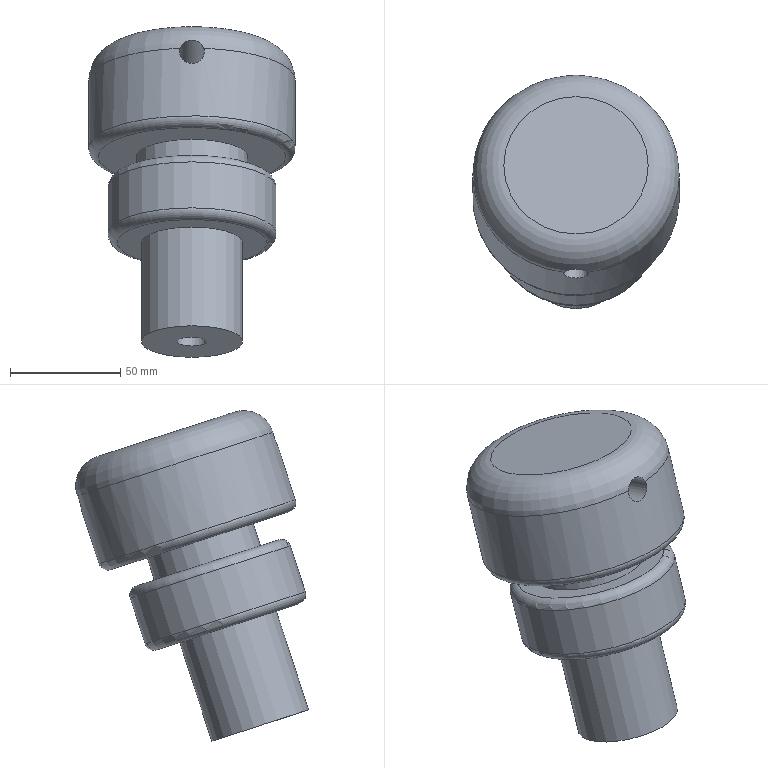Part | NX | features LINKED_BODY 2, DATUM_CSYS 1, Delete Body 1, Resize Face 1 | 1 solid | 19 faces | box 93.696 x 105.756 x 150.047 mm | volume 549540 mm3 | cylinder 9 | plane 6 | torus 4 | commonest cylinder face diameters 13.187 x3 11.25 x2 46.132 x1 50.625 x1 76.469 x1 93.696 x1
STEP:
#1=CARTESIAN_POINT('',(11.25,2935.24,-228.676));
#2=VERTEX_POINT('',#1);
#3=CARTESIAN_POINT('',(11.25,2941.511,-230.713));
#4=DIRECTION('',(0.,0.309,0.9511));
#5=DIRECTION('',(0.,-0.9511,0.309));
#6=AXIS2_PLACEMENT_3D('',#3,#4,#5);
#7=CIRCLE('',#6,6.594);
#8=EDGE_CURVE('',#2,#2,#7,.T.);
#9=ORIENTED_EDGE('',*,*,#8,.F.);
#10=EDGE_LOOP('',(#9));
#11=FACE_BOUND('',#10,.T.);
#12=CARTESIAN_POINT('',(16.87,2976.373,-112.26));
#13=VERTEX_POINT('',#12);
#14=CARTESIAN_POINT('',(5.63,2976.373,-112.26));
#15=VERTEX_POINT('',#14);
#16=CARTESIAN_POINT('',(16.87,2976.373,-112.26));
#17=CARTESIAN_POINT('',(16.904,2976.174,-113.052));
#18=CARTESIAN_POINT('',(16.6,2975.172,-114.385));
#19=CARTESIAN_POINT('',(15.455,2973.427,-115.676));
#20=CARTESIAN_POINT('',(13.683,2971.995,-116.606));
#21=CARTESIAN_POINT('',(11.25,2971.36,-116.988));
#22=CARTESIAN_POINT('',(8.831,2971.988,-116.61));
#23=CARTESIAN_POINT('',(7.045,2973.426,-115.676));
#24=CARTESIAN_POINT('',(5.901,2975.17,-114.39));
#25=CARTESIAN_POINT('',(5.596,2976.175,-113.047));
#26=CARTESIAN_POINT('',(5.63,2976.373,-112.26));
#27=B_SPLINE_CURVE_WITH_KNOTS('',3,(#16,#17,#18,#19,#20,#21,#22,#23,#24,#25,#26),.UNSPECIFIED.,.F.,.F.,(4,1,1,1,1,1,1,1,4),(0.006959,0.009375,0.01179,0.01421,0.01662,0.01904,0.02145,0.02387,0.02629),.UNSPECIFIED.);
#28=EDGE_CURVE('',#13,#15,#27,.T.);
#29=ORIENTED_EDGE('',*,*,#28,.F.);
#30=CARTESIAN_POINT('',(16.87,2982.932,-114.391));
#31=VERTEX_POINT('',#30);
#32=CARTESIAN_POINT('',(11.25,2979.653,-113.326));
#33=DIRECTION('',(0.,0.309,0.9511));
#34=DIRECTION('',(0.,-0.9511,0.309));
#35=AXIS2_PLACEMENT_3D('',#32,#33,#34);
#36=CIRCLE('',#35,6.594);
#37=EDGE_CURVE('',#13,#31,#36,.T.);
#38=ORIENTED_EDGE('',*,*,#37,.T.);
#39=CARTESIAN_POINT('',(5.63,2982.932,-114.391));
#40=VERTEX_POINT('',#39);
#41=CARTESIAN_POINT('',(5.63,2982.932,-114.391));
#42=CARTESIAN_POINT('',(5.596,2982.627,-115.149));
#43=CARTESIAN_POINT('',(5.9,2982.654,-116.816));
#44=CARTESIAN_POINT('',(7.045,2983.308,-118.887));
#45=CARTESIAN_POINT('',(8.817,2983.92,-120.481));
#46=CARTESIAN_POINT('',(11.25,2984.208,-121.163));
#47=CARTESIAN_POINT('',(13.669,2983.922,-120.488));
#48=CARTESIAN_POINT('',(15.455,2983.309,-118.887));
#49=CARTESIAN_POINT('',(16.599,2982.654,-116.822));
#50=CARTESIAN_POINT('',(16.904,2982.63,-115.144));
#51=CARTESIAN_POINT('',(16.87,2982.932,-114.391));
#52=B_SPLINE_CURVE_WITH_KNOTS('',3,(#41,#42,#43,#44,#45,#46,#47,#48,#49,#50,#51),.UNSPECIFIED.,.F.,.F.,(4,1,1,1,1,1,1,1,4),(0.006959,0.009375,0.01179,0.01421,0.01662,0.01904,0.02145,0.02387,0.02629),.UNSPECIFIED.);
#53=EDGE_CURVE('',#40,#31,#52,.T.);
#54=ORIENTED_EDGE('',*,*,#53,.F.);
#55=CARTESIAN_POINT('',(11.25,2979.653,-113.326));
#56=DIRECTION('',(0.,0.309,0.9511));
#57=DIRECTION('',(0.,-0.9511,0.309));
#58=AXIS2_PLACEMENT_3D('',#55,#56,#57);
#59=CIRCLE('',#58,6.594);
#60=EDGE_CURVE('',#40,#15,#59,.T.);
#61=ORIENTED_EDGE('',*,*,#60,.T.);
#62=EDGE_LOOP('',(#29,#38,#54,#61));
#63=FACE_BOUND('',#62,.T.);
#64=CARTESIAN_POINT('',(11.25,2999.02,-53.718));
#65=DIRECTION('',(0.,0.309,0.9511));
#66=DIRECTION('',(0.,-0.9511,0.309));
#67=AXIS2_PLACEMENT_3D('',#64,#65,#66);
#68=CYLINDRICAL_SURFACE('',#67,6.594);
#69=ADVANCED_FACE('',(#11,#63),#68,.F.);
#70=CARTESIAN_POINT('',(11.25,2953.252,-88.483));
#71=VERTEX_POINT('',#70);
#72=CARTESIAN_POINT('',(11.25,2984.433,-98.614));
#73=DIRECTION('',(0.,0.309,0.9511));
#74=DIRECTION('',(0.,-0.9511,0.309));
#75=AXIS2_PLACEMENT_3D('',#72,#73,#74);
#76=CIRCLE('',#75,32.785);
#77=EDGE_CURVE('',#71,#71,#76,.T.);
#78=ORIENTED_EDGE('',*,*,#77,.T.);
#79=EDGE_LOOP('',(#78));
#80=FACE_BOUND('',#79,.T.);
#81=CARTESIAN_POINT('',(11.25,2984.433,-98.614));
#82=DIRECTION('',(0.,0.309,0.9511));
#83=DIRECTION('',(0.,-0.9511,0.309));
#84=AXIS2_PLACEMENT_3D('',#81,#82,#83);
#85=PLANE('',#84);
#86=ADVANCED_FACE('',(#80),#85,.T.);
#87=CARTESIAN_POINT('',(11.25,3014.647,-157.226));
#88=VERTEX_POINT('',#87);
#89=CARTESIAN_POINT('',(11.25,2970.092,-142.749));
#90=DIRECTION('',(0.,-0.309,-0.9511));
#91=DIRECTION('',(0.,0.9511,-0.309));
#92=AXIS2_PLACEMENT_3D('',#89,#90,#91);
#93=CIRCLE('',#92,46.848);
#94=EDGE_CURVE('',#88,#88,#93,.F.);
#95=ORIENTED_EDGE('',*,*,#94,.T.);
#96=EDGE_LOOP('',(#95));
#97=FACE_BOUND('',#96,.T.);
#98=CARTESIAN_POINT('',(16.63,3024.347,-126.369));
#99=VERTEX_POINT('',#98);
#100=CARTESIAN_POINT('',(5.87,3024.347,-126.369));
#101=VERTEX_POINT('',#100);
#102=CARTESIAN_POINT('',(16.63,3024.347,-126.369));
#103=CARTESIAN_POINT('',(17.146,3023.768,-127.959));
#104=CARTESIAN_POINT('',(16.472,3022.703,-131.618));
#105=CARTESIAN_POINT('',(11.248,3022.243,-134.257));
#106=CARTESIAN_POINT('',(6.024,3022.704,-131.611));
#107=CARTESIAN_POINT('',(5.354,3023.768,-127.959));
#108=CARTESIAN_POINT('',(5.87,3024.347,-126.369));
#109=B_SPLINE_CURVE_WITH_KNOTS('',3,(#102,#103,#104,#105,#106,#107,#108),.UNSPECIFIED.,.F.,.F.,(4,1,1,1,4),(0.,0.005231,0.01046,0.01569,0.02093),.UNSPECIFIED.);
#110=EDGE_CURVE('',#99,#101,#109,.T.);
#111=ORIENTED_EDGE('',*,*,#110,.F.);
#112=CARTESIAN_POINT('',(16.63,2935.827,-97.607));
#113=VERTEX_POINT('',#112);
#114=CARTESIAN_POINT('',(11.25,2980.087,-111.988));
#115=DIRECTION('',(0.,0.309,0.9511));
#116=DIRECTION('',(0.,-0.9511,0.309));
#117=AXIS2_PLACEMENT_3D('',#114,#115,#116);
#118=CIRCLE('',#117,46.848);
#119=EDGE_CURVE('',#99,#113,#118,.F.);
#120=ORIENTED_EDGE('',*,*,#119,.T.);
#121=CARTESIAN_POINT('',(5.87,2935.827,-97.607));
#122=VERTEX_POINT('',#121);
#123=CARTESIAN_POINT('',(5.87,2935.827,-97.607));
#124=CARTESIAN_POINT('',(5.354,2935.361,-99.234));
#125=CARTESIAN_POINT('',(6.028,2934.073,-102.82));
#126=CARTESIAN_POINT('',(11.252,2932.893,-105.225));
#127=CARTESIAN_POINT('',(16.476,2934.075,-102.814));
#128=CARTESIAN_POINT('',(17.146,2935.361,-99.234));
#129=CARTESIAN_POINT('',(16.63,2935.827,-97.607));
#130=B_SPLINE_CURVE_WITH_KNOTS('',3,(#123,#124,#125,#126,#127,#128,#129),.UNSPECIFIED.,.F.,.F.,(4,1,1,1,4),(0.,0.005231,0.01046,0.01569,0.02093),.UNSPECIFIED.);
#131=EDGE_CURVE('',#122,#113,#130,.T.);
#132=ORIENTED_EDGE('',*,*,#131,.F.);
#133=CARTESIAN_POINT('',(11.25,2980.087,-111.988));
#134=DIRECTION('',(0.,0.309,0.9511));
#135=DIRECTION('',(0.,-0.9511,0.309));
#136=AXIS2_PLACEMENT_3D('',#133,#134,#135);
#137=CIRCLE('',#136,46.848);
#138=EDGE_CURVE('',#122,#101,#137,.F.);
#139=ORIENTED_EDGE('',*,*,#138,.T.);
#140=EDGE_LOOP('',(#111,#120,#132,#139));
#141=FACE_BOUND('',#140,.T.);
#142=CARTESIAN_POINT('',(11.25,2999.02,-53.718));
#143=DIRECTION('',(0.,0.309,0.9511));
#144=DIRECTION('',(0.,-0.9511,0.309));
#145=AXIS2_PLACEMENT_3D('',#142,#143,#144);
#146=CYLINDRICAL_SURFACE('',#145,46.848);
#147=ADVANCED_FACE('',(#97,#141),#146,.T.);
#148=CARTESIAN_POINT('',(11.25,3009.332,-159.934));
#149=VERTEX_POINT('',#148);
#150=CARTESIAN_POINT('',(11.25,2968.789,-146.761));
#151=DIRECTION('',(0.,-0.309,-0.9511));
#152=DIRECTION('',(0.,0.9511,-0.309));
#153=AXIS2_PLACEMENT_3D('',#150,#151,#152);
#154=CIRCLE('',#153,42.629);
#155=EDGE_CURVE('',#149,#149,#154,.T.);
#156=ORIENTED_EDGE('',*,*,#155,.T.);
#157=EDGE_LOOP('',(#156));
#158=FACE_BOUND('',#157,.T.);
#159=CARTESIAN_POINT('',(11.25,2944.715,-138.939));
#160=VERTEX_POINT('',#159);
#161=CARTESIAN_POINT('',(11.25,2968.789,-146.761));
#162=DIRECTION('',(0.,0.309,0.9511));
#163=DIRECTION('',(0.,-0.9511,0.309));
#164=AXIS2_PLACEMENT_3D('',#161,#162,#163);
#165=CIRCLE('',#164,25.312);
#166=EDGE_CURVE('',#160,#160,#165,.T.);
#167=ORIENTED_EDGE('',*,*,#166,.T.);
#168=EDGE_LOOP('',(#167));
#169=FACE_BOUND('',#168,.T.);
#170=CARTESIAN_POINT('',(11.25,3013.344,-161.238));
#171=DIRECTION('',(0.,-0.309,-0.9511));
#172=DIRECTION('',(0.,0.9511,-0.309));
#173=AXIS2_PLACEMENT_3D('',#170,#171,#172);
#174=PLANE('',#173);
#175=ADVANCED_FACE('',(#158,#169),#174,.T.);
#176=CARTESIAN_POINT('',(11.25,2941.404,-149.13));
#177=VERTEX_POINT('',#176);
#178=CARTESIAN_POINT('',(11.25,2965.477,-156.952));
#179=DIRECTION('',(0.,0.309,0.9511));
#180=DIRECTION('',(0.,-0.9511,0.309));
#181=AXIS2_PLACEMENT_3D('',#178,#179,#180);
#182=CIRCLE('',#181,25.312);
#183=EDGE_CURVE('',#177,#177,#182,.T.);
#184=ORIENTED_EDGE('',*,*,#183,.T.);
#185=EDGE_LOOP('',(#184));
#186=FACE_BOUND('',#185,.T.);
#187=ORIENTED_EDGE('',*,*,#166,.F.);
#188=EDGE_LOOP('',(#187));
#189=FACE_BOUND('',#188,.T.);
#190=CARTESIAN_POINT('',(11.25,2999.02,-53.718));
#191=DIRECTION('',(0.,0.309,0.9511));
#192=DIRECTION('',(0.,-0.9511,0.309));
#193=AXIS2_PLACEMENT_3D('',#190,#191,#192);
#194=CYLINDRICAL_SURFACE('',#193,25.312);
#195=ADVANCED_FACE('',(#186,#189),#194,.T.);
#196=CARTESIAN_POINT('',(11.25,2933.126,-146.441));
#197=VERTEX_POINT('',#196);
#198=CARTESIAN_POINT('',(11.25,2965.477,-156.952));
#199=DIRECTION('',(0.,0.309,0.9511));
#200=DIRECTION('',(0.,-0.9511,0.309));
#201=AXIS2_PLACEMENT_3D('',#198,#199,#200);
#202=CIRCLE('',#201,34.016);
#203=EDGE_CURVE('',#197,#197,#202,.T.);
#204=ORIENTED_EDGE('',*,*,#203,.T.);
#205=EDGE_LOOP('',(#204));
#206=FACE_BOUND('',#205,.T.);
#207=ORIENTED_EDGE('',*,*,#183,.F.);
#208=EDGE_LOOP('',(#207));
#209=FACE_BOUND('',#208,.T.);
#210=CARTESIAN_POINT('',(11.25,2989.551,-164.774));
#211=DIRECTION('',(0.,0.309,0.9511));
#212=DIRECTION('',(0.,-0.9511,0.309));
#213=AXIS2_PLACEMENT_3D('',#210,#211,#212);
#214=PLANE('',#213);
#215=ADVANCED_FACE('',(#206,#209),#214,.T.);
#216=CARTESIAN_POINT('',(11.25,2993.752,-193.664));
#217=VERTEX_POINT('',#216);
#218=CARTESIAN_POINT('',(11.25,2957.388,-181.848));
#219=DIRECTION('',(0.,-0.309,-0.9511));
#220=DIRECTION('',(0.,0.9511,-0.309));
#221=AXIS2_PLACEMENT_3D('',#218,#219,#220);
#222=CIRCLE('',#221,38.235);
#223=EDGE_CURVE('',#217,#217,#222,.F.);
#224=ORIENTED_EDGE('',*,*,#223,.T.);
#225=EDGE_LOOP('',(#224));
#226=FACE_BOUND('',#225,.T.);
#227=CARTESIAN_POINT('',(11.25,2927.81,-149.15));
#228=VERTEX_POINT('',#227);
#229=CARTESIAN_POINT('',(11.25,2964.174,-160.965));
#230=DIRECTION('',(0.,0.309,0.9511));
#231=DIRECTION('',(0.,-0.9511,0.309));
#232=AXIS2_PLACEMENT_3D('',#229,#230,#231);
#233=CIRCLE('',#232,38.235);
#234=EDGE_CURVE('',#228,#228,#233,.F.);
#235=ORIENTED_EDGE('',*,*,#234,.T.);
#236=EDGE_LOOP('',(#235));
#237=FACE_BOUND('',#236,.T.);
#238=CARTESIAN_POINT('',(11.25,2999.02,-53.718));
#239=DIRECTION('',(0.,0.309,0.9511));
#240=DIRECTION('',(0.,-0.9511,0.309));
#241=AXIS2_PLACEMENT_3D('',#238,#239,#240);
#242=CYLINDRICAL_SURFACE('',#241,38.235);
#243=ADVANCED_FACE('',(#226,#237),#242,.T.);
#244=CARTESIAN_POINT('',(11.25,2988.436,-196.372));
#245=VERTEX_POINT('',#244);
#246=CARTESIAN_POINT('',(11.25,2956.085,-185.861));
#247=DIRECTION('',(0.,-0.309,-0.9511));
#248=DIRECTION('',(0.,0.9511,-0.309));
#249=AXIS2_PLACEMENT_3D('',#246,#247,#248);
#250=CIRCLE('',#249,34.016);
#251=EDGE_CURVE('',#245,#245,#250,.T.);
#252=ORIENTED_EDGE('',*,*,#251,.T.);
#253=EDGE_LOOP('',(#252));
#254=FACE_BOUND('',#253,.T.);
#255=CARTESIAN_POINT('',(11.25,2934.148,-178.733));
#256=VERTEX_POINT('',#255);
#257=CARTESIAN_POINT('',(11.25,2956.085,-185.861));
#258=DIRECTION('',(0.,0.309,0.9511));
#259=DIRECTION('',(0.,-0.9511,0.309));
#260=AXIS2_PLACEMENT_3D('',#257,#258,#259);
#261=CIRCLE('',#260,23.066);
#262=EDGE_CURVE('',#256,#256,#261,.T.);
#263=ORIENTED_EDGE('',*,*,#262,.T.);
#264=EDGE_LOOP('',(#263));
#265=FACE_BOUND('',#264,.T.);
#266=CARTESIAN_POINT('',(11.25,2992.448,-197.676));
#267=DIRECTION('',(0.,-0.309,-0.9511));
#268=DIRECTION('',(0.,0.9511,-0.309));
#269=AXIS2_PLACEMENT_3D('',#266,#267,#268);
#270=PLANE('',#269);
#271=ADVANCED_FACE('',(#254,#265),#270,.T.);
#272=CARTESIAN_POINT('',(11.25,2919.574,-223.586));
#273=VERTEX_POINT('',#272);
#274=CARTESIAN_POINT('',(11.25,2941.511,-230.713));
#275=DIRECTION('',(0.,0.309,0.9511));
#276=DIRECTION('',(0.,-0.9511,0.309));
#277=AXIS2_PLACEMENT_3D('',#274,#275,#276);
#278=CIRCLE('',#277,23.066);
#279=EDGE_CURVE('',#273,#273,#278,.T.);
#280=ORIENTED_EDGE('',*,*,#279,.T.);
#281=EDGE_LOOP('',(#280));
#282=FACE_BOUND('',#281,.T.);
#283=ORIENTED_EDGE('',*,*,#262,.F.);
#284=EDGE_LOOP('',(#283));
#285=FACE_BOUND('',#284,.T.);
#286=CARTESIAN_POINT('',(11.25,2999.02,-53.718));
#287=DIRECTION('',(0.,0.309,0.9511));
#288=DIRECTION('',(0.,-0.9511,0.309));
#289=AXIS2_PLACEMENT_3D('',#286,#287,#288);
#290=CYLINDRICAL_SURFACE('',#289,23.066);
#291=ADVANCED_FACE('',(#282,#285),#290,.T.);
#292=ORIENTED_EDGE('',*,*,#8,.T.);
#293=EDGE_LOOP('',(#292));
#294=FACE_BOUND('',#293,.T.);
#295=ORIENTED_EDGE('',*,*,#279,.F.);
#296=EDGE_LOOP('',(#295));
#297=FACE_BOUND('',#296,.T.);
#298=CARTESIAN_POINT('',(11.25,2963.448,-237.841));
#299=DIRECTION('',(0.,-0.309,-0.9511));
#300=DIRECTION('',(0.,0.9511,-0.309));
#301=AXIS2_PLACEMENT_3D('',#298,#299,#300);
#302=PLANE('',#301);
#303=ADVANCED_FACE('',(#294,#297),#302,.T.);
#304=ORIENTED_EDGE('',*,*,#110,.T.);
#305=CARTESIAN_POINT('',(5.87,3024.347,-126.369));
#306=CARTESIAN_POINT('',(6.222,3024.743,-125.284));
#307=CARTESIAN_POINT('',(7.666,3025.234,-123.305));
#308=CARTESIAN_POINT('',(11.244,3025.371,-122.097));
#309=CARTESIAN_POINT('',(14.825,3025.235,-123.296));
#310=CARTESIAN_POINT('',(16.278,3024.743,-125.284));
#311=CARTESIAN_POINT('',(16.63,3024.347,-126.369));
#312=B_SPLINE_CURVE_WITH_KNOTS('',3,(#305,#306,#307,#308,#309,#310,#311),.UNSPECIFIED.,.F.,.F.,(4,1,1,1,4),(0.,0.00357,0.007139,0.01071,0.01428),.UNSPECIFIED.);
#313=EDGE_CURVE('',#101,#99,#312,.T.);
#314=ORIENTED_EDGE('',*,*,#313,.T.);
#315=EDGE_LOOP('',(#304,#314));
#316=FACE_BOUND('',#315,.T.);
#317=CARTESIAN_POINT('',(16.87,2982.932,-114.391));
#318=CARTESIAN_POINT('',(16.838,2983.22,-113.675));
#319=CARTESIAN_POINT('',(16.458,2984.255,-112.51));
#320=CARTESIAN_POINT('',(15.308,2985.879,-111.323));
#321=CARTESIAN_POINT('',(13.558,2987.212,-110.465));
#322=CARTESIAN_POINT('',(11.255,2987.777,-110.123));
#323=CARTESIAN_POINT('',(8.943,2987.213,-110.465));
#324=CARTESIAN_POINT('',(7.196,2985.883,-111.32));
#325=CARTESIAN_POINT('',(6.043,2984.258,-112.507));
#326=CARTESIAN_POINT('',(5.662,2983.22,-113.675));
#327=CARTESIAN_POINT('',(5.63,2982.932,-114.391));
#328=B_SPLINE_CURVE_WITH_KNOTS('',3,(#317,#318,#319,#320,#321,#322,#323,#324,#325,#326,#327),.UNSPECIFIED.,.F.,.F.,(4,1,1,1,1,1,1,1,4),(0.005013,0.007315,0.009617,0.01192,0.01422,0.01652,0.01882,0.02113,0.02343),.UNSPECIFIED.);
#329=EDGE_CURVE('',#31,#40,#328,.T.);
#330=ORIENTED_EDGE('',*,*,#329,.T.);
#331=ORIENTED_EDGE('',*,*,#53,.T.);
#332=EDGE_LOOP('',(#330,#331));
#333=FACE_BOUND('',#332,.T.);
#334=CARTESIAN_POINT('',(11.25,2900.211,-87.761));
#335=DIRECTION('',(0.,-0.9511,0.309));
#336=DIRECTION('',(0.,-0.309,-0.9511));
#337=AXIS2_PLACEMENT_3D('',#334,#335,#336);
#338=CYLINDRICAL_SURFACE('',#337,5.625);
#339=ADVANCED_FACE('',(#316,#333),#338,.F.);
#340=ORIENTED_EDGE('',*,*,#131,.T.);
#341=CARTESIAN_POINT('',(16.63,2935.827,-97.607));
#342=CARTESIAN_POINT('',(16.278,2936.145,-96.497));
#343=CARTESIAN_POINT('',(14.834,2936.911,-94.607));
#344=CARTESIAN_POINT('',(11.256,2937.51,-93.55));
#345=CARTESIAN_POINT('',(7.675,2936.915,-94.599));
#346=CARTESIAN_POINT('',(6.222,2936.145,-96.497));
#347=CARTESIAN_POINT('',(5.87,2935.827,-97.607));
#348=B_SPLINE_CURVE_WITH_KNOTS('',3,(#341,#342,#343,#344,#345,#346,#347),.UNSPECIFIED.,.F.,.F.,(4,1,1,1,4),(0.,0.00357,0.007139,0.01071,0.01428),.UNSPECIFIED.);
#349=EDGE_CURVE('',#113,#122,#348,.T.);
#350=ORIENTED_EDGE('',*,*,#349,.T.);
#351=EDGE_LOOP('',(#340,#350));
#352=FACE_BOUND('',#351,.T.);
#353=CARTESIAN_POINT('',(5.63,2976.373,-112.26));
#354=CARTESIAN_POINT('',(5.662,2976.561,-111.511));
#355=CARTESIAN_POINT('',(6.042,2976.409,-109.961));
#356=CARTESIAN_POINT('',(7.192,2975.792,-108.045));
#357=CARTESIAN_POINT('',(8.942,2975.218,-106.568));
#358=CARTESIAN_POINT('',(11.245,2974.962,-105.959));
#359=CARTESIAN_POINT('',(13.557,2975.218,-106.567));
#360=CARTESIAN_POINT('',(15.304,2975.791,-108.041));
#361=CARTESIAN_POINT('',(16.457,2976.408,-109.957));
#362=CARTESIAN_POINT('',(16.838,2976.561,-111.511));
#363=CARTESIAN_POINT('',(16.87,2976.373,-112.26));
#364=B_SPLINE_CURVE_WITH_KNOTS('',3,(#353,#354,#355,#356,#357,#358,#359,#360,#361,#362,#363),.UNSPECIFIED.,.F.,.F.,(4,1,1,1,1,1,1,1,4),(0.005013,0.007315,0.009617,0.01192,0.01422,0.01652,0.01882,0.02113,0.02343),.UNSPECIFIED.);
#365=EDGE_CURVE('',#15,#13,#364,.T.);
#366=ORIENTED_EDGE('',*,*,#365,.T.);
#367=ORIENTED_EDGE('',*,*,#28,.T.);
#368=EDGE_LOOP('',(#366,#367));
#369=FACE_BOUND('',#368,.T.);
#370=CARTESIAN_POINT('',(11.25,2900.211,-87.761));
#371=DIRECTION('',(0.,-0.9511,0.309));
#372=DIRECTION('',(0.,-0.309,-0.9511));
#373=AXIS2_PLACEMENT_3D('',#370,#371,#372);
#374=CYLINDRICAL_SURFACE('',#373,5.625);
#375=ADVANCED_FACE('',(#352,#369),#374,.F.);
#376=ORIENTED_EDGE('',*,*,#349,.F.);
#377=ORIENTED_EDGE('',*,*,#119,.F.);
#378=ORIENTED_EDGE('',*,*,#313,.F.);
#379=ORIENTED_EDGE('',*,*,#138,.F.);
#380=EDGE_LOOP('',(#376,#377,#378,#379));
#381=FACE_BOUND('',#380,.T.);
#382=ORIENTED_EDGE('',*,*,#77,.F.);
#383=EDGE_LOOP('',(#382));
#384=FACE_BOUND('',#383,.T.);
#385=CARTESIAN_POINT('',(11.25,2980.087,-111.988));
#386=DIRECTION('',(0.,0.309,0.9511));
#387=DIRECTION('',(0.,-0.9511,0.309));
#388=AXIS2_PLACEMENT_3D('',#385,#386,#387);
#389=TOROIDAL_SURFACE('',#388,32.785,14.062);
#390=ADVANCED_FACE('',(#381,#384),#389,.T.);
#391=ORIENTED_EDGE('',*,*,#365,.F.);
#392=CARTESIAN_POINT('',(11.25,2979.653,-113.326));
#393=DIRECTION('',(0.,0.309,0.9511));
#394=DIRECTION('',(0.,-0.9511,0.309));
#395=AXIS2_PLACEMENT_3D('',#392,#393,#394);
#396=CIRCLE('',#395,6.594);
#397=EDGE_CURVE('',#15,#13,#396,.T.);
#398=ORIENTED_EDGE('',*,*,#397,.T.);
#399=EDGE_LOOP('',(#391,#398));
#400=FACE_BOUND('',#399,.T.);
#401=CARTESIAN_POINT('',(11.25,2979.653,-113.326));
#402=DIRECTION('',(0.,0.309,0.9511));
#403=DIRECTION('',(0.,-0.9511,0.309));
#404=AXIS2_PLACEMENT_3D('',#401,#402,#403);
#405=CYLINDRICAL_SURFACE('',#404,6.594);
#406=ADVANCED_FACE('',(#400),#405,.T.);
#407=ORIENTED_EDGE('',*,*,#329,.F.);
#408=CARTESIAN_POINT('',(11.25,2979.653,-113.326));
#409=DIRECTION('',(0.,0.309,0.9511));
#410=DIRECTION('',(0.,-0.9511,0.309));
#411=AXIS2_PLACEMENT_3D('',#408,#409,#410);
#412=CIRCLE('',#411,6.594);
#413=EDGE_CURVE('',#31,#40,#412,.T.);
#414=ORIENTED_EDGE('',*,*,#413,.T.);
#415=EDGE_LOOP('',(#407,#414));
#416=FACE_BOUND('',#415,.T.);
#417=CARTESIAN_POINT('',(11.25,2979.653,-113.326));
#418=DIRECTION('',(0.,0.309,0.9511));
#419=DIRECTION('',(0.,-0.9511,0.309));
#420=AXIS2_PLACEMENT_3D('',#417,#418,#419);
#421=CYLINDRICAL_SURFACE('',#420,6.594);
#422=ADVANCED_FACE('',(#416),#421,.T.);
#423=ORIENTED_EDGE('',*,*,#37,.F.);
#424=ORIENTED_EDGE('',*,*,#397,.F.);
#425=ORIENTED_EDGE('',*,*,#60,.F.);
#426=ORIENTED_EDGE('',*,*,#413,.F.);
#427=EDGE_LOOP('',(#423,#424,#425,#426));
#428=FACE_BOUND('',#427,.T.);
#429=CARTESIAN_POINT('',(11.25,2979.653,-113.326));
#430=DIRECTION('',(0.,0.309,0.9511));
#431=DIRECTION('',(0.,-0.9511,0.309));
#432=AXIS2_PLACEMENT_3D('',#429,#430,#431);
#433=PLANE('',#432);
#434=ADVANCED_FACE('',(#428),#433,.F.);
#435=ORIENTED_EDGE('',*,*,#155,.F.);
#436=EDGE_LOOP('',(#435));
#437=FACE_BOUND('',#436,.T.);
#438=ORIENTED_EDGE('',*,*,#94,.F.);
#439=EDGE_LOOP('',(#438));
#440=FACE_BOUND('',#439,.T.);
#441=CARTESIAN_POINT('',(11.25,2970.092,-142.749));
#442=DIRECTION('',(0.,-0.309,-0.9511));
#443=DIRECTION('',(0.,0.9511,-0.309));
#444=AXIS2_PLACEMENT_3D('',#441,#442,#443);
#445=TOROIDAL_SURFACE('',#444,42.629,4.219);
#446=ADVANCED_FACE('',(#437,#440),#445,.T.);
#447=ORIENTED_EDGE('',*,*,#251,.F.);
#448=EDGE_LOOP('',(#447));
#449=FACE_BOUND('',#448,.T.);
#450=ORIENTED_EDGE('',*,*,#223,.F.);
#451=EDGE_LOOP('',(#450));
#452=FACE_BOUND('',#451,.T.);
#453=CARTESIAN_POINT('',(11.25,2957.388,-181.848));
#454=DIRECTION('',(0.,-0.309,-0.9511));
#455=DIRECTION('',(0.,0.9511,-0.309));
#456=AXIS2_PLACEMENT_3D('',#453,#454,#455);
#457=TOROIDAL_SURFACE('',#456,34.016,4.219);
#458=ADVANCED_FACE('',(#449,#452),#457,.T.);
#459=ORIENTED_EDGE('',*,*,#234,.F.);
#460=EDGE_LOOP('',(#459));
#461=FACE_BOUND('',#460,.T.);
#462=ORIENTED_EDGE('',*,*,#203,.F.);
#463=EDGE_LOOP('',(#462));
#464=FACE_BOUND('',#463,.T.);
#465=CARTESIAN_POINT('',(11.25,2964.174,-160.965));
#466=DIRECTION('',(0.,0.309,0.9511));
#467=DIRECTION('',(0.,-0.9511,0.309));
#468=AXIS2_PLACEMENT_3D('',#465,#466,#467);
#469=TOROIDAL_SURFACE('',#468,34.016,4.219);
#470=ADVANCED_FACE('',(#461,#464),#469,.T.);
#471=CLOSED_SHELL('',(#69,#86,#147,#175,#195,#215,#243,#271,#291,#303,#339,#375,#390,#406,#422,#434,#446,#458,#470));
#472=MANIFOLD_SOLID_BREP('',#471);
#473=(LENGTH_UNIT()NAMED_UNIT(*)SI_UNIT(.MILLI.,.METRE.));
#474=UNCERTAINTY_MEASURE_WITH_UNIT(LENGTH_MEASURE(0.0508),#473,'','');
#475=(NAMED_UNIT(*)PLANE_ANGLE_UNIT()SI_UNIT($,.RADIAN.));
#476=(NAMED_UNIT(*)SI_UNIT($,.STERADIAN.)SOLID_ANGLE_UNIT());
#477=(GEOMETRIC_REPRESENTATION_CONTEXT(3)GLOBAL_UNCERTAINTY_ASSIGNED_CONTEXT((#474))GLOBAL_UNIT_ASSIGNED_CONTEXT((#473,#475,#476))REPRESENTATION_CONTEXT('',''));
#478=ADVANCED_BREP_SHAPE_REPRESENTATION('',(#472),#477);